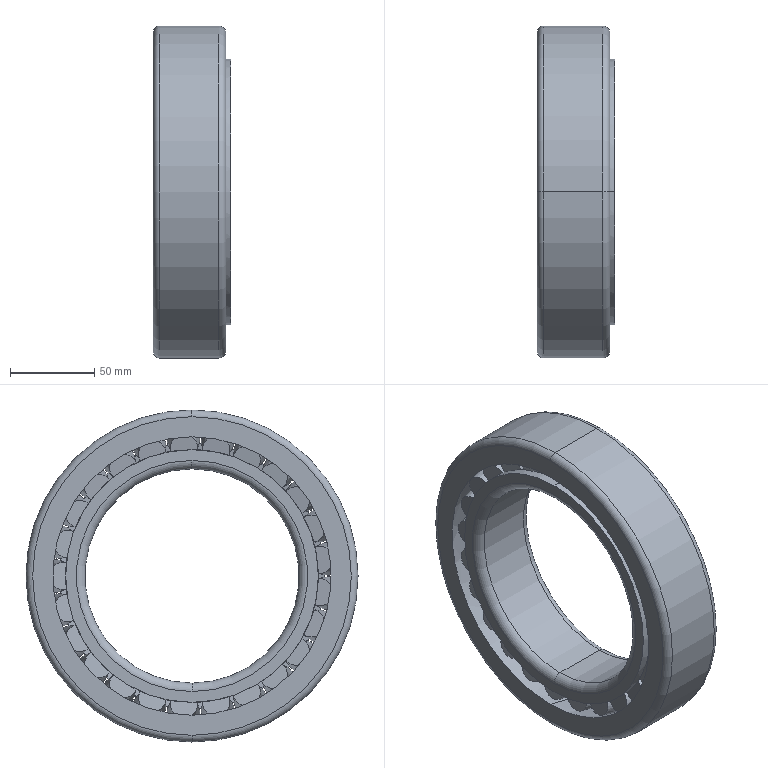Part | SolidWorks | features Revolution 3, Fillet 2, CirPattern 1 | 1 solid | 200 faces | box 46.04 x 196.8 x 196.8 mm | volume 612337 mm3 | cone 130 | plane 54 | torus 8 | cylinder 8 | commonest cylinder face diameters 127 x2 149.8 x2 157.4 x2 196.8 x2